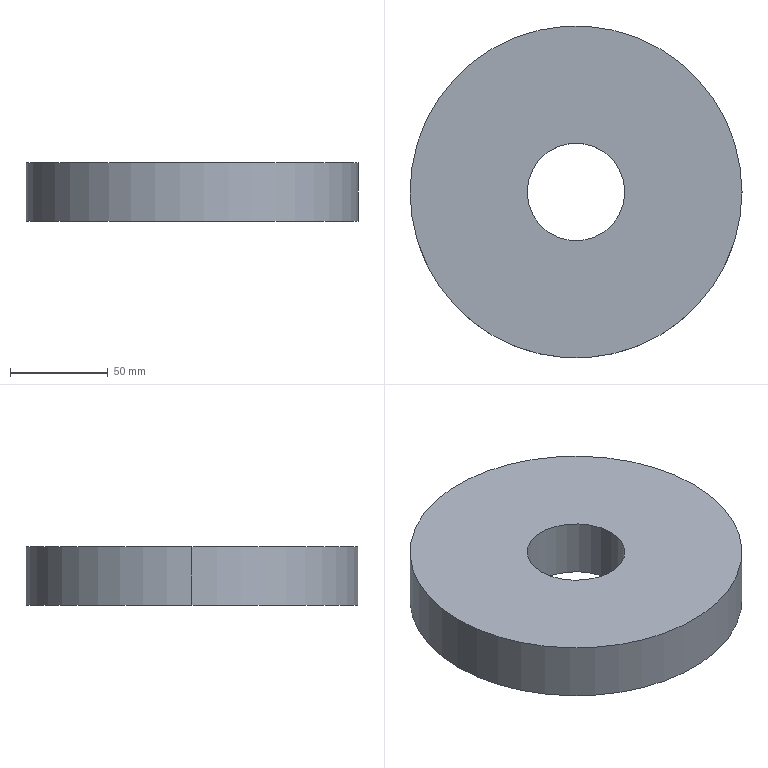Part | SolidWorks | features Extrusion 1 | 1 solid | 6 faces | box 170 x 170 x 30 mm | volume 622035 mm3 | cylinder 4 | plane 2 | commonest cylinder face diameters 50 x2 170 x2
STEP:
#1=CARTESIAN_POINT('',(-25.,0.,30.));
#2=VERTEX_POINT('',#1);
#3=CARTESIAN_POINT('',(25.,0.,30.));
#4=VERTEX_POINT('',#3);
#5=CARTESIAN_POINT('',(0.,0.,30.));
#6=DIRECTION('',(0.,0.,1.));
#7=DIRECTION('',(1.,0.,0.));
#8=AXIS2_PLACEMENT_3D('',#5,#6,#7);
#9=CIRCLE('',#8,25.);
#10=EDGE_CURVE('',#2,#4,#9,.T.);
#11=ORIENTED_EDGE('',*,*,#10,.T.);
#12=CARTESIAN_POINT('',(25.,0.,0.));
#13=VERTEX_POINT('',#12);
#14=CARTESIAN_POINT('',(25.,0.,30.));
#15=DIRECTION('',(0.,0.,-1.));
#16=VECTOR('',#15,1000.);
#17=LINE('',#14,#16);
#18=EDGE_CURVE('',#4,#13,#17,.T.);
#19=ORIENTED_EDGE('',*,*,#18,.T.);
#20=CARTESIAN_POINT('',(-25.,0.,0.));
#21=VERTEX_POINT('',#20);
#22=CARTESIAN_POINT('',(0.,0.,0.));
#23=DIRECTION('',(0.,0.,1.));
#24=DIRECTION('',(1.,0.,0.));
#25=AXIS2_PLACEMENT_3D('',#22,#23,#24);
#26=CIRCLE('',#25,25.);
#27=EDGE_CURVE('',#21,#13,#26,.T.);
#28=ORIENTED_EDGE('',*,*,#27,.F.);
#29=CARTESIAN_POINT('',(-25.,0.,30.));
#30=DIRECTION('',(0.,0.,-1.));
#31=VECTOR('',#30,1000.);
#32=LINE('',#29,#31);
#33=EDGE_CURVE('',#2,#21,#32,.T.);
#34=ORIENTED_EDGE('',*,*,#33,.F.);
#35=EDGE_LOOP('',(#11,#19,#28,#34));
#36=FACE_OUTER_BOUND('',#35,.T.);
#37=CARTESIAN_POINT('',(0.,0.,30.));
#38=DIRECTION('',(0.,0.,-1.));
#39=DIRECTION('',(-1.,0.,0.));
#40=AXIS2_PLACEMENT_3D('',#37,#38,#39);
#41=CYLINDRICAL_SURFACE('',#40,25.);
#42=ADVANCED_FACE('',(#36),#41,.F.);
#43=CARTESIAN_POINT('',(85.,0.,30.));
#44=VERTEX_POINT('',#43);
#45=CARTESIAN_POINT('',(-85.,0.,30.));
#46=VERTEX_POINT('',#45);
#47=CARTESIAN_POINT('',(0.,0.,30.));
#48=DIRECTION('',(0.,0.,1.));
#49=DIRECTION('',(1.,0.,0.));
#50=AXIS2_PLACEMENT_3D('',#47,#48,#49);
#51=CIRCLE('',#50,85.);
#52=EDGE_CURVE('',#44,#46,#51,.T.);
#53=ORIENTED_EDGE('',*,*,#52,.F.);
#54=CARTESIAN_POINT('',(85.,0.,0.));
#55=VERTEX_POINT('',#54);
#56=CARTESIAN_POINT('',(85.,0.,30.));
#57=DIRECTION('',(0.,0.,-1.));
#58=VECTOR('',#57,1000.);
#59=LINE('',#56,#58);
#60=EDGE_CURVE('',#44,#55,#59,.T.);
#61=ORIENTED_EDGE('',*,*,#60,.T.);
#62=CARTESIAN_POINT('',(-85.,0.,0.));
#63=VERTEX_POINT('',#62);
#64=CARTESIAN_POINT('',(0.,0.,0.));
#65=DIRECTION('',(0.,0.,1.));
#66=DIRECTION('',(1.,0.,0.));
#67=AXIS2_PLACEMENT_3D('',#64,#65,#66);
#68=CIRCLE('',#67,85.);
#69=EDGE_CURVE('',#55,#63,#68,.T.);
#70=ORIENTED_EDGE('',*,*,#69,.T.);
#71=CARTESIAN_POINT('',(-85.,0.,30.));
#72=DIRECTION('',(0.,0.,-1.));
#73=VECTOR('',#72,1000.);
#74=LINE('',#71,#73);
#75=EDGE_CURVE('',#46,#63,#74,.T.);
#76=ORIENTED_EDGE('',*,*,#75,.F.);
#77=EDGE_LOOP('',(#53,#61,#70,#76));
#78=FACE_OUTER_BOUND('',#77,.T.);
#79=CARTESIAN_POINT('',(0.,0.,30.));
#80=DIRECTION('',(0.,0.,-1.));
#81=DIRECTION('',(-1.,0.,0.));
#82=AXIS2_PLACEMENT_3D('',#79,#80,#81);
#83=CYLINDRICAL_SURFACE('',#82,85.);
#84=ADVANCED_FACE('',(#78),#83,.T.);
#85=CARTESIAN_POINT('',(0.,0.,30.));
#86=DIRECTION('',(0.,0.,1.));
#87=DIRECTION('',(1.,0.,0.));
#88=AXIS2_PLACEMENT_3D('',#85,#86,#87);
#89=CIRCLE('',#88,85.);
#90=EDGE_CURVE('',#46,#44,#89,.T.);
#91=ORIENTED_EDGE('',*,*,#90,.T.);
#92=ORIENTED_EDGE('',*,*,#52,.T.);
#93=EDGE_LOOP('',(#91,#92));
#94=FACE_OUTER_BOUND('',#93,.T.);
#95=ORIENTED_EDGE('',*,*,#10,.F.);
#96=CARTESIAN_POINT('',(0.,0.,30.));
#97=DIRECTION('',(0.,0.,1.));
#98=DIRECTION('',(1.,0.,0.));
#99=AXIS2_PLACEMENT_3D('',#96,#97,#98);
#100=CIRCLE('',#99,25.);
#101=EDGE_CURVE('',#4,#2,#100,.T.);
#102=ORIENTED_EDGE('',*,*,#101,.F.);
#103=EDGE_LOOP('',(#95,#102));
#104=FACE_BOUND('',#103,.T.);
#105=CARTESIAN_POINT('',(0.,0.,30.));
#106=DIRECTION('',(0.,0.,1.));
#107=DIRECTION('',(1.,0.,0.));
#108=AXIS2_PLACEMENT_3D('',#105,#106,#107);
#109=PLANE('',#108);
#110=ADVANCED_FACE('',(#94,#104),#109,.T.);
#111=CARTESIAN_POINT('',(0.,0.,0.));
#112=DIRECTION('',(0.,0.,1.));
#113=DIRECTION('',(1.,0.,0.));
#114=AXIS2_PLACEMENT_3D('',#111,#112,#113);
#115=CIRCLE('',#114,85.);
#116=EDGE_CURVE('',#63,#55,#115,.T.);
#117=ORIENTED_EDGE('',*,*,#116,.F.);
#118=ORIENTED_EDGE('',*,*,#69,.F.);
#119=EDGE_LOOP('',(#117,#118));
#120=FACE_OUTER_BOUND('',#119,.T.);
#121=ORIENTED_EDGE('',*,*,#27,.T.);
#122=CARTESIAN_POINT('',(0.,0.,0.));
#123=DIRECTION('',(0.,0.,1.));
#124=DIRECTION('',(1.,0.,0.));
#125=AXIS2_PLACEMENT_3D('',#122,#123,#124);
#126=CIRCLE('',#125,25.);
#127=EDGE_CURVE('',#13,#21,#126,.T.);
#128=ORIENTED_EDGE('',*,*,#127,.T.);
#129=EDGE_LOOP('',(#121,#128));
#130=FACE_BOUND('',#129,.T.);
#131=CARTESIAN_POINT('',(0.,0.,0.));
#132=DIRECTION('',(0.,0.,1.));
#133=DIRECTION('',(1.,0.,0.));
#134=AXIS2_PLACEMENT_3D('',#131,#132,#133);
#135=PLANE('',#134);
#136=ADVANCED_FACE('',(#120,#130),#135,.F.);
#137=ORIENTED_EDGE('',*,*,#60,.F.);
#138=ORIENTED_EDGE('',*,*,#90,.F.);
#139=ORIENTED_EDGE('',*,*,#75,.T.);
#140=ORIENTED_EDGE('',*,*,#116,.T.);
#141=EDGE_LOOP('',(#137,#138,#139,#140));
#142=FACE_OUTER_BOUND('',#141,.T.);
#143=CARTESIAN_POINT('',(0.,0.,30.));
#144=DIRECTION('',(0.,0.,-1.));
#145=DIRECTION('',(-1.,0.,0.));
#146=AXIS2_PLACEMENT_3D('',#143,#144,#145);
#147=CYLINDRICAL_SURFACE('',#146,85.);
#148=ADVANCED_FACE('',(#142),#147,.T.);
#149=ORIENTED_EDGE('',*,*,#18,.F.);
#150=ORIENTED_EDGE('',*,*,#101,.T.);
#151=ORIENTED_EDGE('',*,*,#33,.T.);
#152=ORIENTED_EDGE('',*,*,#127,.F.);
#153=EDGE_LOOP('',(#149,#150,#151,#152));
#154=FACE_OUTER_BOUND('',#153,.T.);
#155=CARTESIAN_POINT('',(0.,0.,30.));
#156=DIRECTION('',(0.,0.,-1.));
#157=DIRECTION('',(-1.,0.,0.));
#158=AXIS2_PLACEMENT_3D('',#155,#156,#157);
#159=CYLINDRICAL_SURFACE('',#158,25.);
#160=ADVANCED_FACE('',(#154),#159,.F.);
#161=CLOSED_SHELL('',(#42,#84,#110,#136,#148,#160));
#162=MANIFOLD_SOLID_BREP('',#161);
#163=CARTESIAN_POINT('',(0.,0.,0.));
#164=DIRECTION('',(0.,0.,1.));
#165=DIRECTION('',(1.,0.,0.));
#166=AXIS2_PLACEMENT_3D('',#163,#164,#165);
#167=(LENGTH_UNIT()NAMED_UNIT(*)SI_UNIT(.MILLI.,.METRE.));
#168=UNCERTAINTY_MEASURE_WITH_UNIT(LENGTH_MEASURE(0.00001),#167,'','');
#169=(NAMED_UNIT(*)PLANE_ANGLE_UNIT()SI_UNIT($,.RADIAN.));
#170=(NAMED_UNIT(*)SI_UNIT($,.STERADIAN.)SOLID_ANGLE_UNIT());
#171=(GEOMETRIC_REPRESENTATION_CONTEXT(3)GLOBAL_UNCERTAINTY_ASSIGNED_CONTEXT((#168))GLOBAL_UNIT_ASSIGNED_CONTEXT((#167,#169,#170))REPRESENTATION_CONTEXT('',''));
#172=ADVANCED_BREP_SHAPE_REPRESENTATION('',(#162,#166),#171);